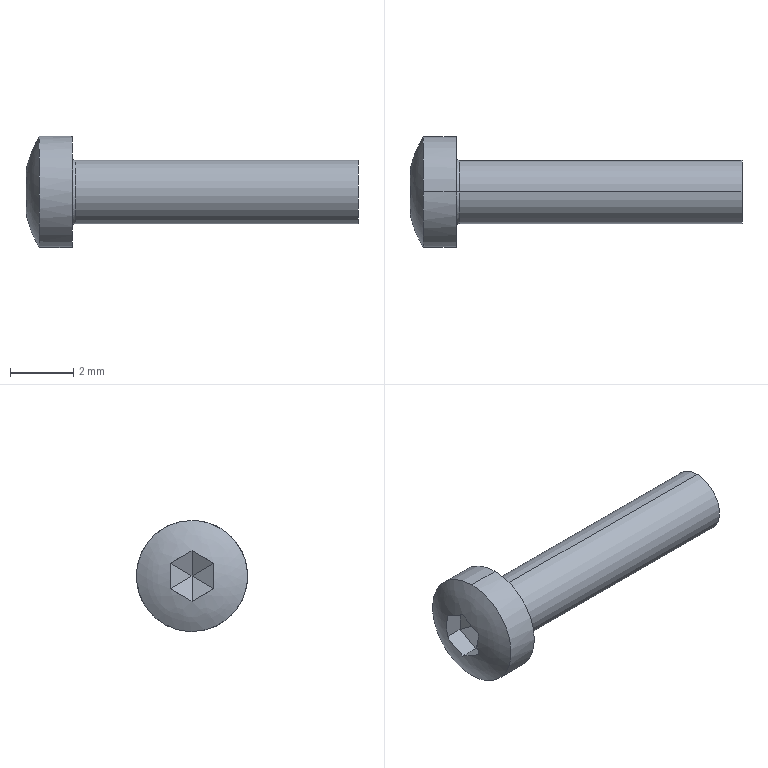Part | SolidWorks | features BaseBody 1, ICE 1, MoveFace 1, Scale 1 | 1 solid | 21 faces | box 10.461 x 3.5 x 3.5 mm | volume 39.454 mm3 | plane 14 | cylinder 4 | spline 3 | commonest cylinder face diameters 2 x2 3.5 x2
STEP:
#1=CARTESIAN_POINT('',(1.533,0.,1.083));
#2=VERTEX_POINT('',#1);
#3=CARTESIAN_POINT('',(1.533,0.,-1.083));
#4=VERTEX_POINT('',#3);
#5=CARTESIAN_POINT('',(1.533,0.,1.083));
#6=CARTESIAN_POINT('',(1.533,0.06885,1.083));
#7=CARTESIAN_POINT('',(1.533,0.1703,1.074));
#8=CARTESIAN_POINT('',(1.533,0.2856,1.046));
#9=CARTESIAN_POINT('',(1.533,0.3343,1.031));
#10=CARTESIAN_POINT('',(1.533,0.3667,1.02));
#11=CARTESIAN_POINT('',(1.533,0.3814,1.014));
#12=CARTESIAN_POINT('',(1.533,0.5377,0.9523));
#13=CARTESIAN_POINT('',(1.533,0.6603,0.8717));
#14=CARTESIAN_POINT('',(1.533,0.8189,0.7132));
#15=CARTESIAN_POINT('',(1.533,0.8887,0.6277));
#16=CARTESIAN_POINT('',(1.533,0.9535,0.5169));
#17=CARTESIAN_POINT('',(1.533,0.9777,0.467));
#18=CARTESIAN_POINT('',(1.533,0.9931,0.4333));
#19=CARTESIAN_POINT('',(1.533,1.001,0.4148));
#20=CARTESIAN_POINT('',(1.533,1.058,0.2708));
#21=CARTESIAN_POINT('',(1.533,1.083,0.1376));
#22=CARTESIAN_POINT('',(1.533,1.083,-0.06882));
#23=CARTESIAN_POINT('',(1.533,1.074,-0.1703));
#24=CARTESIAN_POINT('',(1.533,1.046,-0.2856));
#25=CARTESIAN_POINT('',(1.533,1.031,-0.3343));
#26=CARTESIAN_POINT('',(1.533,1.02,-0.3666));
#27=CARTESIAN_POINT('',(1.533,1.014,-0.3814));
#28=CARTESIAN_POINT('',(1.533,0.9523,-0.5377));
#29=CARTESIAN_POINT('',(1.533,0.8717,-0.6603));
#30=CARTESIAN_POINT('',(1.533,0.7132,-0.8189));
#31=CARTESIAN_POINT('',(1.533,0.6277,-0.8887));
#32=CARTESIAN_POINT('',(1.533,0.5169,-0.9535));
#33=CARTESIAN_POINT('',(1.533,0.467,-0.9777));
#34=CARTESIAN_POINT('',(1.533,0.4333,-0.9931));
#35=CARTESIAN_POINT('',(1.533,0.4148,-1.001));
#36=CARTESIAN_POINT('',(1.533,0.2707,-1.058));
#37=CARTESIAN_POINT('',(1.533,0.1378,-1.083));
#38=CARTESIAN_POINT('',(1.533,0.,-1.083));
#39=B_SPLINE_CURVE_WITH_KNOTS('',3,(#5,#6,#7,#8,#9,#10,#11,#12,#13,#14,#15,#16,#17,#18,#19,#20,#21,#22,#23,#24,#25,#26,#27,#28,#29,#30,#31,#32,#33,#34,#35,#36,#37,#38),.UNSPECIFIED.,.F.,.F.,(4,1,1,2,2,2,1,1,2,2,2,1,1,2,2,2,1,1,2,2,4),(0.,0.0625,0.09375,0.1094,0.125,0.25,0.3125,0.3437,0.3594,0.375,0.5,0.5625,0.5937,0.6094,0.625,0.75,0.8125,0.8437,0.8594,0.875,1.),.UNSPECIFIED.);
#40=EDGE_CURVE('',#2,#4,#39,.T.);
#41=ORIENTED_EDGE('',*,*,#40,.F.);
#42=CARTESIAN_POINT('',(1.617,0.,1.));
#43=VERTEX_POINT('',#42);
#44=CARTESIAN_POINT('',(1.617,0.,1.083));
#45=DIRECTION('',(0.,-1.,0.));
#46=DIRECTION('',(0.,0.,1.));
#47=AXIS2_PLACEMENT_3D('',#44,#45,#46);
#48=CIRCLE('',#47,0.08333);
#49=EDGE_CURVE('',#2,#43,#48,.T.);
#50=ORIENTED_EDGE('',*,*,#49,.T.);
#51=CARTESIAN_POINT('',(1.617,0.,-1.));
#52=VERTEX_POINT('',#51);
#53=CARTESIAN_POINT('',(1.617,0.,0.));
#54=DIRECTION('',(1.,0.,0.));
#55=DIRECTION('',(0.,0.,1.));
#56=AXIS2_PLACEMENT_3D('',#53,#54,#55);
#57=CIRCLE('',#56,1.);
#58=EDGE_CURVE('',#52,#43,#57,.T.);
#59=ORIENTED_EDGE('',*,*,#58,.F.);
#60=CARTESIAN_POINT('',(1.617,0.,-1.083));
#61=DIRECTION('',(0.,1.,0.));
#62=DIRECTION('',(0.,0.,-1.));
#63=AXIS2_PLACEMENT_3D('',#60,#61,#62);
#64=CIRCLE('',#63,0.08333);
#65=EDGE_CURVE('',#4,#52,#64,.T.);
#66=ORIENTED_EDGE('',*,*,#65,.F.);
#67=EDGE_LOOP('',(#41,#50,#59,#66));
#68=FACE_OUTER_BOUND('',#67,.T.);
#69=CARTESIAN_POINT('',(1.533,0.,-1.083));
#70=CARTESIAN_POINT('',(1.533,2.167,-1.083));
#71=CARTESIAN_POINT('',(1.533,2.167,1.083));
#72=CARTESIAN_POINT('',(1.533,0.,1.083));
#73=CARTESIAN_POINT('',(1.533,0.,-1.035));
#74=CARTESIAN_POINT('',(1.533,2.069,-1.035));
#75=CARTESIAN_POINT('',(1.533,2.069,1.035));
#76=CARTESIAN_POINT('',(1.533,0.,1.035));
#77=CARTESIAN_POINT('',(1.568,0.,-1.));
#78=CARTESIAN_POINT('',(1.568,2.,-1.));
#79=CARTESIAN_POINT('',(1.568,2.,1.));
#80=CARTESIAN_POINT('',(1.568,0.,1.));
#81=CARTESIAN_POINT('',(1.617,0.,-1.));
#82=CARTESIAN_POINT('',(1.617,2.,-1.));
#83=CARTESIAN_POINT('',(1.617,2.,1.));
#84=CARTESIAN_POINT('',(1.617,0.,1.));
#85=(BOUNDED_SURFACE()B_SPLINE_SURFACE(3,3,((#69,#70,#71,#72),(#73,#74,#75,#76),(#77,#78,#79,#80),(#81,#82,#83,#84)),.UNSPECIFIED.,.F.,.F.,.F.)B_SPLINE_SURFACE_WITH_KNOTS((4,4),(4,4),(0.,1.),(0.,1.),.UNSPECIFIED.)GEOMETRIC_REPRESENTATION_ITEM()RATIONAL_B_SPLINE_SURFACE(((1.,0.3333,0.3333,1.),(0.8047,0.2682,0.2682,0.8047),(0.8047,0.2682,0.2682,0.8047),(1.,0.3333,0.3333,1.)))REPRESENTATION_ITEM('')SURFACE());
#86=ADVANCED_FACE('',(#68),#85,.F.);
#87=CARTESIAN_POINT('',(0.4963,0.,1.75));
#88=VERTEX_POINT('',#87);
#89=CARTESIAN_POINT('',(0.4963,0.,-1.75));
#90=VERTEX_POINT('',#89);
#91=CARTESIAN_POINT('',(0.4963,0.,1.75));
#92=CARTESIAN_POINT('',(0.4963,0.2284,1.75));
#93=CARTESIAN_POINT('',(0.4963,0.4585,1.704));
#94=CARTESIAN_POINT('',(0.4963,0.8798,1.53));
#95=CARTESIAN_POINT('',(0.4963,1.075,1.4));
#96=CARTESIAN_POINT('',(0.4963,1.317,1.158));
#97=CARTESIAN_POINT('',(0.4963,1.391,1.068));
#98=CARTESIAN_POINT('',(0.4963,1.518,0.8775));
#99=CARTESIAN_POINT('',(0.4963,1.572,0.777));
#100=CARTESIAN_POINT('',(0.4963,1.66,0.5654));
#101=CARTESIAN_POINT('',(0.4963,1.694,0.4541));
#102=CARTESIAN_POINT('',(0.4963,1.739,0.2304));
#103=CARTESIAN_POINT('',(0.4963,1.75,0.1169));
#104=CARTESIAN_POINT('',(0.4963,1.75,-0.2293));
#105=CARTESIAN_POINT('',(0.4963,1.705,-0.4565));
#106=CARTESIAN_POINT('',(0.4963,1.573,-0.7749));
#107=CARTESIAN_POINT('',(0.4963,1.52,-0.8754));
#108=CARTESIAN_POINT('',(0.4963,1.393,-1.066));
#109=CARTESIAN_POINT('',(0.4963,1.319,-1.156));
#110=CARTESIAN_POINT('',(0.4963,1.077,-1.398));
#111=CARTESIAN_POINT('',(0.4963,0.8819,-1.529));
#112=CARTESIAN_POINT('',(0.4963,0.4609,-1.704));
#113=CARTESIAN_POINT('',(0.4963,0.2312,-1.75));
#114=CARTESIAN_POINT('',(0.4963,0.,-1.75));
#115=B_SPLINE_CURVE_WITH_KNOTS('',3,(#91,#92,#93,#94,#95,#96,#97,#98,#99,#100,#101,#102,#103,#104,#105,#106,#107,#108,#109,#110,#111,#112,#113,#114),.UNSPECIFIED.,.F.,.F.,(4,2,2,2,2,2,2,2,2,2,2,4),(0.005471,0.006155,0.006839,0.007181,0.007523,0.007864,0.008206,0.00889,0.009232,0.009574,0.01026,0.01094),.UNSPECIFIED.);
#116=EDGE_CURVE('',#88,#90,#115,.T.);
#117=ORIENTED_EDGE('',*,*,#116,.F.);
#118=CARTESIAN_POINT('',(1.533,0.,1.75));
#119=VERTEX_POINT('',#118);
#120=CARTESIAN_POINT('',(-0.02526,0.,1.75));
#121=DIRECTION('',(1.,0.,0.));
#122=VECTOR('',#121,1000.);
#123=LINE('',#120,#122);
#124=EDGE_CURVE('',#88,#119,#123,.T.);
#125=ORIENTED_EDGE('',*,*,#124,.T.);
#126=CARTESIAN_POINT('',(1.533,0.,-1.75));
#127=VERTEX_POINT('',#126);
#128=CARTESIAN_POINT('',(1.533,0.,0.));
#129=DIRECTION('',(1.,0.,0.));
#130=DIRECTION('',(0.,0.,-1.));
#131=AXIS2_PLACEMENT_3D('',#128,#129,#130);
#132=CIRCLE('',#131,1.75);
#133=EDGE_CURVE('',#127,#119,#132,.T.);
#134=ORIENTED_EDGE('',*,*,#133,.F.);
#135=CARTESIAN_POINT('',(-0.02526,0.,-1.75));
#136=DIRECTION('',(1.,0.,0.));
#137=VECTOR('',#136,1000.);
#138=LINE('',#135,#137);
#139=EDGE_CURVE('',#90,#127,#138,.T.);
#140=ORIENTED_EDGE('',*,*,#139,.F.);
#141=EDGE_LOOP('',(#117,#125,#134,#140));
#142=FACE_OUTER_BOUND('',#141,.T.);
#143=CARTESIAN_POINT('',(-0.02526,0.,0.));
#144=DIRECTION('',(1.,0.,0.));
#145=DIRECTION('',(0.,0.,-1.));
#146=AXIS2_PLACEMENT_3D('',#143,#144,#145);
#147=CYLINDRICAL_SURFACE('',#146,1.75);
#148=ADVANCED_FACE('',(#142),#147,.T.);
#149=CARTESIAN_POINT('',(10.533,0.,1.));
#150=VERTEX_POINT('',#149);
#151=CARTESIAN_POINT('',(10.533,0.,-1.));
#152=VERTEX_POINT('',#151);
#153=CARTESIAN_POINT('',(10.533,0.,0.));
#154=DIRECTION('',(-1.,0.,0.));
#155=DIRECTION('',(0.,0.,1.));
#156=AXIS2_PLACEMENT_3D('',#153,#154,#155);
#157=CIRCLE('',#156,1.);
#158=EDGE_CURVE('',#150,#152,#157,.T.);
#159=ORIENTED_EDGE('',*,*,#158,.T.);
#160=CARTESIAN_POINT('',(5.533,0.,-1.));
#161=DIRECTION('',(-1.,0.,0.));
#162=VECTOR('',#161,1000.);
#163=LINE('',#160,#162);
#164=EDGE_CURVE('',#152,#52,#163,.T.);
#165=ORIENTED_EDGE('',*,*,#164,.T.);
#166=ORIENTED_EDGE('',*,*,#58,.T.);
#167=CARTESIAN_POINT('',(5.533,0.,1.));
#168=DIRECTION('',(-1.,0.,0.));
#169=VECTOR('',#168,1000.);
#170=LINE('',#167,#169);
#171=EDGE_CURVE('',#150,#43,#170,.T.);
#172=ORIENTED_EDGE('',*,*,#171,.F.);
#173=EDGE_LOOP('',(#159,#165,#166,#172));
#174=FACE_OUTER_BOUND('',#173,.T.);
#175=CARTESIAN_POINT('',(5.533,0.,0.));
#176=DIRECTION('',(-1.,0.,0.));
#177=DIRECTION('',(0.,0.,1.));
#178=AXIS2_PLACEMENT_3D('',#175,#176,#177);
#179=CYLINDRICAL_SURFACE('',#178,1.);
#180=ADVANCED_FACE('',(#174),#179,.T.);
#181=CARTESIAN_POINT('',(1.533,0.,-1.083));
#182=CARTESIAN_POINT('',(1.533,-0.06885,-1.083));
#183=CARTESIAN_POINT('',(1.533,-0.1703,-1.074));
#184=CARTESIAN_POINT('',(1.533,-0.2856,-1.046));
#185=CARTESIAN_POINT('',(1.533,-0.3343,-1.031));
#186=CARTESIAN_POINT('',(1.533,-0.3667,-1.02));
#187=CARTESIAN_POINT('',(1.533,-0.3814,-1.014));
#188=CARTESIAN_POINT('',(1.533,-0.5377,-0.9523));
#189=CARTESIAN_POINT('',(1.533,-0.6603,-0.8717));
#190=CARTESIAN_POINT('',(1.533,-0.8189,-0.7132));
#191=CARTESIAN_POINT('',(1.533,-0.8887,-0.6277));
#192=CARTESIAN_POINT('',(1.533,-0.9535,-0.5169));
#193=CARTESIAN_POINT('',(1.533,-0.9777,-0.467));
#194=CARTESIAN_POINT('',(1.533,-0.9931,-0.4333));
#195=CARTESIAN_POINT('',(1.533,-1.001,-0.4148));
#196=CARTESIAN_POINT('',(1.533,-1.058,-0.2708));
#197=CARTESIAN_POINT('',(1.533,-1.083,-0.1376));
#198=CARTESIAN_POINT('',(1.533,-1.083,0.06882));
#199=CARTESIAN_POINT('',(1.533,-1.074,0.1703));
#200=CARTESIAN_POINT('',(1.533,-1.046,0.2856));
#201=CARTESIAN_POINT('',(1.533,-1.031,0.3343));
#202=CARTESIAN_POINT('',(1.533,-1.02,0.3666));
#203=CARTESIAN_POINT('',(1.533,-1.014,0.3814));
#204=CARTESIAN_POINT('',(1.533,-0.9523,0.5377));
#205=CARTESIAN_POINT('',(1.533,-0.8717,0.6603));
#206=CARTESIAN_POINT('',(1.533,-0.7132,0.8189));
#207=CARTESIAN_POINT('',(1.533,-0.6277,0.8887));
#208=CARTESIAN_POINT('',(1.533,-0.5169,0.9535));
#209=CARTESIAN_POINT('',(1.533,-0.467,0.9777));
#210=CARTESIAN_POINT('',(1.533,-0.4333,0.9931));
#211=CARTESIAN_POINT('',(1.533,-0.4148,1.001));
#212=CARTESIAN_POINT('',(1.533,-0.2707,1.058));
#213=CARTESIAN_POINT('',(1.533,-0.1378,1.083));
#214=CARTESIAN_POINT('',(1.533,0.,1.083));
#215=B_SPLINE_CURVE_WITH_KNOTS('',3,(#181,#182,#183,#184,#185,#186,#187,#188,#189,#190,#191,#192,#193,#194,#195,#196,#197,#198,#199,#200,#201,#202,#203,#204,#205,#206,#207,#208,#209,#210,#211,#212,#213,#214),.UNSPECIFIED.,.F.,.F.,(4,1,1,2,2,2,1,1,2,2,2,1,1,2,2,2,1,1,2,2,4),(0.,0.0625,0.09375,0.1094,0.125,0.25,0.3125,0.3438,0.3594,0.375,0.5,0.5625,0.5938,0.6094,0.625,0.75,0.8125,0.8438,0.8594,0.875,1.),.UNSPECIFIED.);
#216=EDGE_CURVE('',#4,#2,#215,.T.);
#217=ORIENTED_EDGE('',*,*,#216,.T.);
#218=ORIENTED_EDGE('',*,*,#40,.T.);
#219=EDGE_LOOP('',(#217,#218));
#220=FACE_BOUND('',#219,.T.);
#221=ORIENTED_EDGE('',*,*,#133,.T.);
#222=CARTESIAN_POINT('',(1.533,0.,0.));
#223=DIRECTION('',(1.,0.,0.));
#224=DIRECTION('',(0.,0.,-1.));
#225=AXIS2_PLACEMENT_3D('',#222,#223,#224);
#226=CIRCLE('',#225,1.75);
#227=EDGE_CURVE('',#119,#127,#226,.T.);
#228=ORIENTED_EDGE('',*,*,#227,.T.);
#229=EDGE_LOOP('',(#221,#228));
#230=FACE_OUTER_BOUND('',#229,.T.);
#231=CARTESIAN_POINT('',(1.533,0.,0.));
#232=DIRECTION('',(1.,0.,0.));
#233=DIRECTION('',(0.,0.,-1.));
#234=AXIS2_PLACEMENT_3D('',#231,#232,#233);
#235=PLANE('',#234);
#236=ADVANCED_FACE('',(#220,#230),#235,.T.);
#237=ORIENTED_EDGE('',*,*,#164,.F.);
#238=CARTESIAN_POINT('',(10.533,0.,0.));
#239=DIRECTION('',(-1.,0.,0.));
#240=DIRECTION('',(0.,0.,1.));
#241=AXIS2_PLACEMENT_3D('',#238,#239,#240);
#242=CIRCLE('',#241,1.);
#243=EDGE_CURVE('',#152,#150,#242,.T.);
#244=ORIENTED_EDGE('',*,*,#243,.T.);
#245=ORIENTED_EDGE('',*,*,#171,.T.);
#246=CARTESIAN_POINT('',(1.617,0.,0.));
#247=DIRECTION('',(1.,0.,0.));
#248=DIRECTION('',(0.,0.,1.));
#249=AXIS2_PLACEMENT_3D('',#246,#247,#248);
#250=CIRCLE('',#249,1.);
#251=EDGE_CURVE('',#43,#52,#250,.T.);
#252=ORIENTED_EDGE('',*,*,#251,.T.);
#253=EDGE_LOOP('',(#237,#244,#245,#252));
#254=FACE_OUTER_BOUND('',#253,.T.);
#255=CARTESIAN_POINT('',(5.533,0.,0.));
#256=DIRECTION('',(-1.,0.,0.));
#257=DIRECTION('',(0.,0.,1.));
#258=AXIS2_PLACEMENT_3D('',#255,#256,#257);
#259=CYLINDRICAL_SURFACE('',#258,1.);
#260=ADVANCED_FACE('',(#254),#259,.T.);
#261=ORIENTED_EDGE('',*,*,#49,.F.);
#262=ORIENTED_EDGE('',*,*,#216,.F.);
#263=ORIENTED_EDGE('',*,*,#65,.T.);
#264=ORIENTED_EDGE('',*,*,#251,.F.);
#265=EDGE_LOOP('',(#261,#262,#263,#264));
#266=FACE_OUTER_BOUND('',#265,.T.);
#267=CARTESIAN_POINT('',(1.533,0.,1.083));
#268=CARTESIAN_POINT('',(1.533,-2.167,1.083));
#269=CARTESIAN_POINT('',(1.533,-2.167,-1.083));
#270=CARTESIAN_POINT('',(1.533,0.,-1.083));
#271=CARTESIAN_POINT('',(1.533,0.,1.035));
#272=CARTESIAN_POINT('',(1.533,-2.069,1.035));
#273=CARTESIAN_POINT('',(1.533,-2.069,-1.035));
#274=CARTESIAN_POINT('',(1.533,0.,-1.035));
#275=CARTESIAN_POINT('',(1.568,0.,1.));
#276=CARTESIAN_POINT('',(1.568,-2.,1.));
#277=CARTESIAN_POINT('',(1.568,-2.,-1.));
#278=CARTESIAN_POINT('',(1.568,0.,-1.));
#279=CARTESIAN_POINT('',(1.617,0.,1.));
#280=CARTESIAN_POINT('',(1.617,-2.,1.));
#281=CARTESIAN_POINT('',(1.617,-2.,-1.));
#282=CARTESIAN_POINT('',(1.617,0.,-1.));
#283=(BOUNDED_SURFACE()B_SPLINE_SURFACE(3,3,((#267,#268,#269,#270),(#271,#272,#273,#274),(#275,#276,#277,#278),(#279,#280,#281,#282)),.UNSPECIFIED.,.F.,.F.,.F.)B_SPLINE_SURFACE_WITH_KNOTS((4,4),(4,4),(0.,1.),(0.,1.),.UNSPECIFIED.)GEOMETRIC_REPRESENTATION_ITEM()RATIONAL_B_SPLINE_SURFACE(((1.,0.3333,0.3333,1.),(0.8047,0.2682,0.2682,0.8047),(0.8047,0.2682,0.2682,0.8047),(1.,0.3333,0.3333,1.)))REPRESENTATION_ITEM('')SURFACE());
#284=ADVANCED_FACE('',(#266),#283,.F.);
#285=ORIENTED_EDGE('',*,*,#158,.F.);
#286=ORIENTED_EDGE('',*,*,#243,.F.);
#287=EDGE_LOOP('',(#285,#286));
#288=FACE_OUTER_BOUND('',#287,.T.);
#289=CARTESIAN_POINT('',(10.533,0.,0.));
#290=DIRECTION('',(1.,0.,0.));
#291=DIRECTION('',(0.,0.,-1.));
#292=AXIS2_PLACEMENT_3D('',#289,#290,#291);
#293=PLANE('',#292);
#294=ADVANCED_FACE('',(#288),#293,.T.);
#295=ORIENTED_EDGE('',*,*,#124,.F.);
#296=CARTESIAN_POINT('',(0.4963,0.,-1.75));
#297=CARTESIAN_POINT('',(0.4963,-0.1156,-1.75));
#298=CARTESIAN_POINT('',(0.4963,-0.2293,-1.739));
#299=CARTESIAN_POINT('',(0.4963,-0.453,-1.694));
#300=CARTESIAN_POINT('',(0.4963,-0.5641,-1.661));
#301=CARTESIAN_POINT('',(0.4963,-0.7761,-1.573));
#302=CARTESIAN_POINT('',(0.4963,-0.8766,-1.519));
#303=CARTESIAN_POINT('',(0.4963,-1.067,-1.392));
#304=CARTESIAN_POINT('',(0.4963,-1.157,-1.318));
#305=CARTESIAN_POINT('',(0.4963,-1.399,-1.076));
#306=CARTESIAN_POINT('',(0.4963,-1.529,-0.8804));
#307=CARTESIAN_POINT('',(0.4963,-1.704,-0.4592));
#308=CARTESIAN_POINT('',(0.4963,-1.75,-0.2289));
#309=CARTESIAN_POINT('',(0.4963,-1.75,0.1135));
#310=CARTESIAN_POINT('',(0.4963,-1.739,0.2295));
#311=CARTESIAN_POINT('',(0.4963,-1.694,0.4539));
#312=CARTESIAN_POINT('',(0.4963,-1.661,0.563));
#313=CARTESIAN_POINT('',(0.4963,-1.573,0.7749));
#314=CARTESIAN_POINT('',(0.4963,-1.518,0.8774));
#315=CARTESIAN_POINT('',(0.4963,-1.392,1.067));
#316=CARTESIAN_POINT('',(0.4963,-1.319,1.155));
#317=CARTESIAN_POINT('',(0.4963,-1.156,1.319));
#318=CARTESIAN_POINT('',(0.4963,-1.067,1.391));
#319=CARTESIAN_POINT('',(0.4963,-0.8779,1.518));
#320=CARTESIAN_POINT('',(0.4963,-0.7757,1.573));
#321=CARTESIAN_POINT('',(0.4963,-0.5635,1.661));
#322=CARTESIAN_POINT('',(0.4963,-0.4544,1.694));
#323=CARTESIAN_POINT('',(0.4963,-0.2302,1.739));
#324=CARTESIAN_POINT('',(0.4963,-0.1142,1.75));
#325=CARTESIAN_POINT('',(0.4963,0.,1.75));
#326=B_SPLINE_CURVE_WITH_KNOTS('',3,(#296,#297,#298,#299,#300,#301,#302,#303,#304,#305,#306,#307,#308,#309,#310,#311,#312,#313,#314,#315,#316,#317,#318,#319,#320,#321,#322,#323,#324,#325),.UNSPECIFIED.,.F.,.F.,(4,2,2,2,2,2,2,2,2,2,2,2,2,2,4),(0.,0.000342,0.0006839,0.001026,0.001368,0.002052,0.002736,0.003078,0.00342,0.003762,0.004103,0.004445,0.004787,0.005129,0.005471),.UNSPECIFIED.);
#327=EDGE_CURVE('',#90,#88,#326,.T.);
#328=ORIENTED_EDGE('',*,*,#327,.F.);
#329=ORIENTED_EDGE('',*,*,#139,.T.);
#330=ORIENTED_EDGE('',*,*,#227,.F.);
#331=EDGE_LOOP('',(#295,#328,#329,#330));
#332=FACE_OUTER_BOUND('',#331,.T.);
#333=CARTESIAN_POINT('',(-0.02526,0.,0.));
#334=DIRECTION('',(1.,0.,0.));
#335=DIRECTION('',(0.,0.,-1.));
#336=AXIS2_PLACEMENT_3D('',#333,#334,#335);
#337=CYLINDRICAL_SURFACE('',#336,1.75);
#338=ADVANCED_FACE('',(#332),#337,.T.);
#339=CARTESIAN_POINT('',(1.066,0.,0.));
#340=VERTEX_POINT('',#339);
#341=CARTESIAN_POINT('',(0.6667,-0.6917,-0.3993));
#342=VERTEX_POINT('',#341);
#343=CARTESIAN_POINT('',(1.066,0.,0.));
#344=DIRECTION('',(-0.4472,-0.7746,-0.4472));
#345=VECTOR('',#344,1000.);
#346=LINE('',#343,#345);
#347=EDGE_CURVE('',#340,#342,#346,.T.);
#348=ORIENTED_EDGE('',*,*,#347,.F.);
#349=CARTESIAN_POINT('',(0.6667,0.,-0.7987));
#350=VERTEX_POINT('',#349);
#351=CARTESIAN_POINT('',(0.6667,0.,-0.7987));
#352=DIRECTION('',(-0.4472,0.,-0.8944));
#353=VECTOR('',#352,1000.);
#354=LINE('',#351,#353);
#355=EDGE_CURVE('',#340,#350,#354,.T.);
#356=ORIENTED_EDGE('',*,*,#355,.T.);
#357=CARTESIAN_POINT('',(0.6667,-0.6917,-0.3993));
#358=DIRECTION('',(0.,0.866,-0.5));
#359=VECTOR('',#358,1000.);
#360=LINE('',#357,#359);
#361=EDGE_CURVE('',#342,#350,#360,.T.);
#362=ORIENTED_EDGE('',*,*,#361,.F.);
#363=EDGE_LOOP('',(#348,#356,#362));
#364=FACE_OUTER_BOUND('',#363,.T.);
#365=CARTESIAN_POINT('',(0.6667,-0.6917,-0.3993));
#366=DIRECTION('',(0.866,-0.25,-0.433));
#367=DIRECTION('',(-0.4472,0.,-0.8944));
#368=AXIS2_PLACEMENT_3D('',#365,#366,#367);
#369=PLANE('',#368);
#370=ADVANCED_FACE('',(#364),#369,.F.);
#371=CARTESIAN_POINT('',(0.6667,-0.6917,0.3993));
#372=VERTEX_POINT('',#371);
#373=CARTESIAN_POINT('',(0.6667,-0.6917,0.3993));
#374=DIRECTION('',(0.4472,0.7746,-0.4472));
#375=VECTOR('',#374,1000.);
#376=LINE('',#373,#375);
#377=EDGE_CURVE('',#372,#340,#376,.T.);
#378=ORIENTED_EDGE('',*,*,#377,.T.);
#379=ORIENTED_EDGE('',*,*,#347,.T.);
#380=CARTESIAN_POINT('',(0.6667,-0.6917,0.3993));
#381=DIRECTION('',(0.,0.,-1.));
#382=VECTOR('',#381,1000.);
#383=LINE('',#380,#382);
#384=EDGE_CURVE('',#372,#342,#383,.T.);
#385=ORIENTED_EDGE('',*,*,#384,.F.);
#386=EDGE_LOOP('',(#378,#379,#385));
#387=FACE_OUTER_BOUND('',#386,.T.);
#388=CARTESIAN_POINT('',(0.6667,-0.6917,0.3993));
#389=DIRECTION('',(0.866,-0.5,0.));
#390=DIRECTION('',(0.5,0.866,0.));
#391=AXIS2_PLACEMENT_3D('',#388,#389,#390);
#392=PLANE('',#391);
#393=ADVANCED_FACE('',(#387),#392,.F.);
#394=CARTESIAN_POINT('',(0.6667,0.,0.7987));
#395=VERTEX_POINT('',#394);
#396=CARTESIAN_POINT('',(0.6667,0.,0.7987));
#397=DIRECTION('',(-0.4472,0.,0.8944));
#398=VECTOR('',#397,1000.);
#399=LINE('',#396,#398);
#400=EDGE_CURVE('',#340,#395,#399,.T.);
#401=ORIENTED_EDGE('',*,*,#400,.F.);
#402=ORIENTED_EDGE('',*,*,#377,.F.);
#403=CARTESIAN_POINT('',(0.6667,0.,0.7987));
#404=DIRECTION('',(0.,-0.866,-0.5));
#405=VECTOR('',#404,1000.);
#406=LINE('',#403,#405);
#407=EDGE_CURVE('',#395,#372,#406,.T.);
#408=ORIENTED_EDGE('',*,*,#407,.F.);
#409=EDGE_LOOP('',(#401,#402,#408));
#410=FACE_OUTER_BOUND('',#409,.T.);
#411=CARTESIAN_POINT('',(0.6667,0.,0.7987));
#412=DIRECTION('',(0.866,-0.25,0.433));
#413=DIRECTION('',(0.4472,0.,-0.8944));
#414=AXIS2_PLACEMENT_3D('',#411,#412,#413);
#415=PLANE('',#414);
#416=ADVANCED_FACE('',(#410),#415,.F.);
#417=CARTESIAN_POINT('',(0.6667,0.6917,0.3993));
#418=VERTEX_POINT('',#417);
#419=CARTESIAN_POINT('',(1.066,0.,0.));
#420=DIRECTION('',(-0.4472,0.7746,0.4472));
#421=VECTOR('',#420,1000.);
#422=LINE('',#419,#421);
#423=EDGE_CURVE('',#340,#418,#422,.T.);
#424=ORIENTED_EDGE('',*,*,#423,.F.);
#425=ORIENTED_EDGE('',*,*,#400,.T.);
#426=CARTESIAN_POINT('',(0.6667,0.6917,0.3993));
#427=DIRECTION('',(0.,-0.866,0.5));
#428=VECTOR('',#427,1000.);
#429=LINE('',#426,#428);
#430=EDGE_CURVE('',#418,#395,#429,.T.);
#431=ORIENTED_EDGE('',*,*,#430,.F.);
#432=EDGE_LOOP('',(#424,#425,#431));
#433=FACE_OUTER_BOUND('',#432,.T.);
#434=CARTESIAN_POINT('',(0.6667,0.6917,0.3993));
#435=DIRECTION('',(0.866,0.25,0.433));
#436=DIRECTION('',(0.4472,0.,-0.8944));
#437=AXIS2_PLACEMENT_3D('',#434,#435,#436);
#438=PLANE('',#437);
#439=ADVANCED_FACE('',(#433),#438,.F.);
#440=CARTESIAN_POINT('',(0.6667,0.6917,-0.3993));
#441=VERTEX_POINT('',#440);
#442=CARTESIAN_POINT('',(0.6667,0.6917,-0.3993));
#443=DIRECTION('',(0.4472,-0.7746,0.4472));
#444=VECTOR('',#443,1000.);
#445=LINE('',#442,#444);
#446=EDGE_CURVE('',#441,#340,#445,.T.);
#447=ORIENTED_EDGE('',*,*,#446,.T.);
#448=ORIENTED_EDGE('',*,*,#423,.T.);
#449=CARTESIAN_POINT('',(0.6667,0.6917,-0.3993));
#450=DIRECTION('',(0.,0.,1.));
#451=VECTOR('',#450,1000.);
#452=LINE('',#449,#451);
#453=EDGE_CURVE('',#441,#418,#452,.T.);
#454=ORIENTED_EDGE('',*,*,#453,.F.);
#455=EDGE_LOOP('',(#447,#448,#454));
#456=FACE_OUTER_BOUND('',#455,.T.);
#457=CARTESIAN_POINT('',(0.6667,0.6917,-0.3993));
#458=DIRECTION('',(0.866,0.5,0.));
#459=DIRECTION('',(-0.5,0.866,0.));
#460=AXIS2_PLACEMENT_3D('',#457,#458,#459);
#461=PLANE('',#460);
#462=ADVANCED_FACE('',(#456),#461,.F.);
#463=ORIENTED_EDGE('',*,*,#355,.F.);
#464=ORIENTED_EDGE('',*,*,#446,.F.);
#465=CARTESIAN_POINT('',(0.6667,0.,-0.7987));
#466=DIRECTION('',(0.,0.866,0.5));
#467=VECTOR('',#466,1000.);
#468=LINE('',#465,#467);
#469=EDGE_CURVE('',#350,#441,#468,.T.);
#470=ORIENTED_EDGE('',*,*,#469,.F.);
#471=EDGE_LOOP('',(#463,#464,#470));
#472=FACE_OUTER_BOUND('',#471,.T.);
#473=CARTESIAN_POINT('',(0.6667,0.,-0.7987));
#474=DIRECTION('',(0.866,0.25,-0.433));
#475=DIRECTION('',(-0.4472,0.,-0.8944));
#476=AXIS2_PLACEMENT_3D('',#473,#474,#475);
#477=PLANE('',#476);
#478=ADVANCED_FACE('',(#472),#477,.F.);
#479=CARTESIAN_POINT('',(0.09709,0.,-0.7987));
#480=VERTEX_POINT('',#479);
#481=CARTESIAN_POINT('',(0.6667,0.,-0.7987));
#482=DIRECTION('',(1.,0.,0.));
#483=VECTOR('',#482,1000.);
#484=LINE('',#481,#483);
#485=EDGE_CURVE('',#480,#350,#484,.T.);
#486=ORIENTED_EDGE('',*,*,#485,.F.);
#487=CARTESIAN_POINT('',(0.09709,-0.6917,-0.3993));
#488=VERTEX_POINT('',#487);
#489=CARTESIAN_POINT('',(0.09709,-0.6917,-0.3993));
#490=CARTESIAN_POINT('',(0.06424,-0.4611,-0.5324));
#491=CARTESIAN_POINT('',(0.06424,-0.2306,-0.6656));
#492=CARTESIAN_POINT('',(0.09709,0.,-0.7987));
#493=B_SPLINE_CURVE_WITH_KNOTS('',3,(#489,#490,#491,#492),.UNSPECIFIED.,.F.,.F.,(4,4),(0.,0.0007987),.UNSPECIFIED.);
#494=EDGE_CURVE('',#488,#480,#493,.T.);
#495=ORIENTED_EDGE('',*,*,#494,.F.);
#496=CARTESIAN_POINT('',(0.6667,-0.6917,-0.3993));
#497=DIRECTION('',(-1.,0.,0.));
#498=VECTOR('',#497,1000.);
#499=LINE('',#496,#498);
#500=EDGE_CURVE('',#342,#488,#499,.T.);
#501=ORIENTED_EDGE('',*,*,#500,.F.);
#502=ORIENTED_EDGE('',*,*,#361,.T.);
#503=EDGE_LOOP('',(#486,#495,#501,#502));
#504=FACE_OUTER_BOUND('',#503,.T.);
#505=CARTESIAN_POINT('',(0.6667,-0.6917,-0.3993));
#506=DIRECTION('',(0.,0.5,0.866));
#507=DIRECTION('',(0.,-0.866,0.5));
#508=AXIS2_PLACEMENT_3D('',#505,#506,#507);
#509=PLANE('',#508);
#510=ADVANCED_FACE('',(#504),#509,.T.);
#511=ORIENTED_EDGE('',*,*,#500,.T.);
#512=CARTESIAN_POINT('',(0.09709,-0.6917,0.3993));
#513=VERTEX_POINT('',#512);
#514=CARTESIAN_POINT('',(3.333,-0.6917,0.));
#515=DIRECTION('',(0.,1.,0.));
#516=DIRECTION('',(0.,0.,-1.));
#517=AXIS2_PLACEMENT_3D('',#514,#515,#516);
#518=CIRCLE('',#517,3.261);
#519=EDGE_CURVE('',#488,#513,#518,.T.);
#520=ORIENTED_EDGE('',*,*,#519,.T.);
#521=CARTESIAN_POINT('',(0.6667,-0.6917,0.3993));
#522=DIRECTION('',(1.,0.,0.));
#523=VECTOR('',#522,1000.);
#524=LINE('',#521,#523);
#525=EDGE_CURVE('',#513,#372,#524,.T.);
#526=ORIENTED_EDGE('',*,*,#525,.T.);
#527=ORIENTED_EDGE('',*,*,#384,.T.);
#528=EDGE_LOOP('',(#511,#520,#526,#527));
#529=FACE_OUTER_BOUND('',#528,.T.);
#530=CARTESIAN_POINT('',(0.6667,-0.6917,0.3993));
#531=DIRECTION('',(0.,1.,0.));
#532=DIRECTION('',(0.,0.,1.));
#533=AXIS2_PLACEMENT_3D('',#530,#531,#532);
#534=PLANE('',#533);
#535=ADVANCED_FACE('',(#529),#534,.T.);
#536=ORIENTED_EDGE('',*,*,#525,.F.);
#537=CARTESIAN_POINT('',(0.09709,0.,0.7987));
#538=VERTEX_POINT('',#537);
#539=CARTESIAN_POINT('',(0.09709,0.,0.7987));
#540=CARTESIAN_POINT('',(0.06424,-0.2306,0.6656));
#541=CARTESIAN_POINT('',(0.06424,-0.4611,0.5324));
#542=CARTESIAN_POINT('',(0.09709,-0.6917,0.3993));
#543=B_SPLINE_CURVE_WITH_KNOTS('',3,(#539,#540,#541,#542),.UNSPECIFIED.,.F.,.F.,(4,4),(0.,0.0007987),.UNSPECIFIED.);
#544=EDGE_CURVE('',#538,#513,#543,.T.);
#545=ORIENTED_EDGE('',*,*,#544,.F.);
#546=CARTESIAN_POINT('',(0.6667,0.,0.7987));
#547=DIRECTION('',(1.,0.,0.));
#548=VECTOR('',#547,1000.);
#549=LINE('',#546,#548);
#550=EDGE_CURVE('',#538,#395,#549,.T.);
#551=ORIENTED_EDGE('',*,*,#550,.T.);
#552=ORIENTED_EDGE('',*,*,#407,.T.);
#553=EDGE_LOOP('',(#536,#545,#551,#552));
#554=FACE_OUTER_BOUND('',#553,.T.);
#555=CARTESIAN_POINT('',(0.6667,0.,0.7987));
#556=DIRECTION('',(0.,0.5,-0.866));
#557=DIRECTION('',(0.,0.866,0.5));
#558=AXIS2_PLACEMENT_3D('',#555,#556,#557);
#559=PLANE('',#558);
#560=ADVANCED_FACE('',(#554),#559,.T.);
#561=ORIENTED_EDGE('',*,*,#550,.F.);
#562=CARTESIAN_POINT('',(0.09709,0.6917,0.3993));
#563=VERTEX_POINT('',#562);
#564=CARTESIAN_POINT('',(0.09709,0.6917,0.3993));
#565=CARTESIAN_POINT('',(0.06424,0.4611,0.5324));
#566=CARTESIAN_POINT('',(0.06424,0.2306,0.6656));
#567=CARTESIAN_POINT('',(0.09709,0.,0.7987));
#568=B_SPLINE_CURVE_WITH_KNOTS('',3,(#564,#565,#566,#567),.UNSPECIFIED.,.F.,.F.,(4,4),(0.,0.0007987),.UNSPECIFIED.);
#569=EDGE_CURVE('',#563,#538,#568,.T.);
#570=ORIENTED_EDGE('',*,*,#569,.F.);
#571=CARTESIAN_POINT('',(0.6667,0.6917,0.3993));
#572=DIRECTION('',(-1.,0.,0.));
#573=VECTOR('',#572,1000.);
#574=LINE('',#571,#573);
#575=EDGE_CURVE('',#418,#563,#574,.T.);
#576=ORIENTED_EDGE('',*,*,#575,.F.);
#577=ORIENTED_EDGE('',*,*,#430,.T.);
#578=EDGE_LOOP('',(#561,#570,#576,#577));
#579=FACE_OUTER_BOUND('',#578,.T.);
#580=CARTESIAN_POINT('',(0.6667,0.6917,0.3993));
#581=DIRECTION('',(0.,-0.5,-0.866));
#582=DIRECTION('',(0.,0.866,-0.5));
#583=AXIS2_PLACEMENT_3D('',#580,#581,#582);
#584=PLANE('',#583);
#585=ADVANCED_FACE('',(#579),#584,.T.);
#586=ORIENTED_EDGE('',*,*,#575,.T.);
#587=CARTESIAN_POINT('',(0.09709,0.6917,-0.3993));
#588=VERTEX_POINT('',#587);
#589=CARTESIAN_POINT('',(3.333,0.6917,0.));
#590=DIRECTION('',(0.,-1.,0.));
#591=DIRECTION('',(0.,0.,-1.));
#592=AXIS2_PLACEMENT_3D('',#589,#590,#591);
#593=CIRCLE('',#592,3.261);
#594=EDGE_CURVE('',#563,#588,#593,.T.);
#595=ORIENTED_EDGE('',*,*,#594,.T.);
#596=CARTESIAN_POINT('',(0.6667,0.6917,-0.3993));
#597=DIRECTION('',(1.,0.,0.));
#598=VECTOR('',#597,1000.);
#599=LINE('',#596,#598);
#600=EDGE_CURVE('',#588,#441,#599,.T.);
#601=ORIENTED_EDGE('',*,*,#600,.T.);
#602=ORIENTED_EDGE('',*,*,#453,.T.);
#603=EDGE_LOOP('',(#586,#595,#601,#602));
#604=FACE_OUTER_BOUND('',#603,.T.);
#605=CARTESIAN_POINT('',(0.6667,0.6917,-0.3993));
#606=DIRECTION('',(0.,-1.,0.));
#607=DIRECTION('',(0.,0.,-1.));
#608=AXIS2_PLACEMENT_3D('',#605,#606,#607);
#609=PLANE('',#608);
#610=ADVANCED_FACE('',(#604),#609,.T.);
#611=ORIENTED_EDGE('',*,*,#600,.F.);
#612=CARTESIAN_POINT('',(0.09709,0.,-0.7987));
#613=CARTESIAN_POINT('',(0.06424,0.2306,-0.6656));
#614=CARTESIAN_POINT('',(0.06424,0.4611,-0.5324));
#615=CARTESIAN_POINT('',(0.09709,0.6917,-0.3993));
#616=B_SPLINE_CURVE_WITH_KNOTS('',3,(#612,#613,#614,#615),.UNSPECIFIED.,.F.,.F.,(4,4),(0.,0.0007987),.UNSPECIFIED.);
#617=EDGE_CURVE('',#480,#588,#616,.T.);
#618=ORIENTED_EDGE('',*,*,#617,.F.);
#619=ORIENTED_EDGE('',*,*,#485,.T.);
#620=ORIENTED_EDGE('',*,*,#469,.T.);
#621=EDGE_LOOP('',(#611,#618,#619,#620));
#622=FACE_OUTER_BOUND('',#621,.T.);
#623=CARTESIAN_POINT('',(0.6667,0.,-0.7987));
#624=DIRECTION('',(0.,-0.5,0.866));
#625=DIRECTION('',(0.,-0.866,-0.5));
#626=AXIS2_PLACEMENT_3D('',#623,#624,#625);
#627=PLANE('',#626);
#628=ADVANCED_FACE('',(#622),#627,.T.);
#629=ORIENTED_EDGE('',*,*,#617,.T.);
#630=ORIENTED_EDGE('',*,*,#594,.F.);
#631=ORIENTED_EDGE('',*,*,#569,.T.);
#632=ORIENTED_EDGE('',*,*,#544,.T.);
#633=ORIENTED_EDGE('',*,*,#519,.F.);
#634=ORIENTED_EDGE('',*,*,#494,.T.);
#635=EDGE_LOOP('',(#629,#630,#631,#632,#633,#634));
#636=FACE_BOUND('',#635,.T.);
#637=ORIENTED_EDGE('',*,*,#327,.T.);
#638=ORIENTED_EDGE('',*,*,#116,.T.);
#639=EDGE_LOOP('',(#637,#638));
#640=FACE_OUTER_BOUND('',#639,.T.);
#641=CARTESIAN_POINT('',(0.9486,-1.78,1.502));
#642=CARTESIAN_POINT('',(0.3554,-1.78,0.5606));
#643=CARTESIAN_POINT('',(0.3538,-1.78,-0.5523));
#644=CARTESIAN_POINT('',(0.9444,-1.78,-1.496));
#645=CARTESIAN_POINT('',(0.353,-0.6648,1.878));
#646=CARTESIAN_POINT('',(-0.3884,-0.6648,0.7007));
#647=CARTESIAN_POINT('',(-0.3904,-0.6648,-0.6903));
#648=CARTESIAN_POINT('',(0.3477,-0.6648,-1.869));
#649=CARTESIAN_POINT('',(0.3512,0.6538,1.879));
#650=CARTESIAN_POINT('',(-0.3906,0.6538,0.7011));
#651=CARTESIAN_POINT('',(-0.3925,0.6538,-0.6907));
#652=CARTESIAN_POINT('',(0.346,0.6538,-1.87));
#653=CARTESIAN_POINT('',(0.9439,1.771,1.505));
#654=CARTESIAN_POINT('',(0.3495,1.771,0.5617));
#655=CARTESIAN_POINT('',(0.348,1.771,-0.5534));
#656=CARTESIAN_POINT('',(0.9397,1.771,-1.499));
#657=(BOUNDED_SURFACE()B_SPLINE_SURFACE(3,3,((#641,#642,#643,#644),(#645,#646,#647,#648),(#649,#650,#651,#652),(#653,#654,#655,#656)),.UNSPECIFIED.,.F.,.F.,.T.)B_SPLINE_SURFACE_WITH_KNOTS((4,4),(4,4),(0.,1.),(0.,1.),.UNSPECIFIED.)GEOMETRIC_REPRESENTATION_ITEM()RATIONAL_B_SPLINE_SURFACE(((1.,0.8979,0.8979,1.),(0.8976,0.8059,0.8059,0.8976),(0.8976,0.8059,0.8059,0.8976),(1.,0.8979,0.8979,1.)))REPRESENTATION_ITEM('')SURFACE());
#658=ADVANCED_FACE('',(#636,#640),#657,.T.);
#659=CLOSED_SHELL('',(#86,#148,#180,#236,#260,#284,#294,#338,#370,#393,#416,#439,#462,#478,#510,#535,#560,#585,#610,#628,#658));
#660=MANIFOLD_SOLID_BREP('',#659);
#661=CARTESIAN_POINT('',(0.,0.,0.));
#662=DIRECTION('',(0.,0.,1.));
#663=DIRECTION('',(1.,0.,0.));
#664=AXIS2_PLACEMENT_3D('',#661,#662,#663);
#665=(LENGTH_UNIT()NAMED_UNIT(*)SI_UNIT(.MILLI.,.METRE.));
#666=UNCERTAINTY_MEASURE_WITH_UNIT(LENGTH_MEASURE(0.00001),#665,'','');
#667=(NAMED_UNIT(*)PLANE_ANGLE_UNIT()SI_UNIT($,.RADIAN.));
#668=(NAMED_UNIT(*)SI_UNIT($,.STERADIAN.)SOLID_ANGLE_UNIT());
#669=(GEOMETRIC_REPRESENTATION_CONTEXT(3)GLOBAL_UNCERTAINTY_ASSIGNED_CONTEXT((#666))GLOBAL_UNIT_ASSIGNED_CONTEXT((#665,#667,#668))REPRESENTATION_CONTEXT('',''));
#670=ADVANCED_BREP_SHAPE_REPRESENTATION('',(#660,#664),#669);